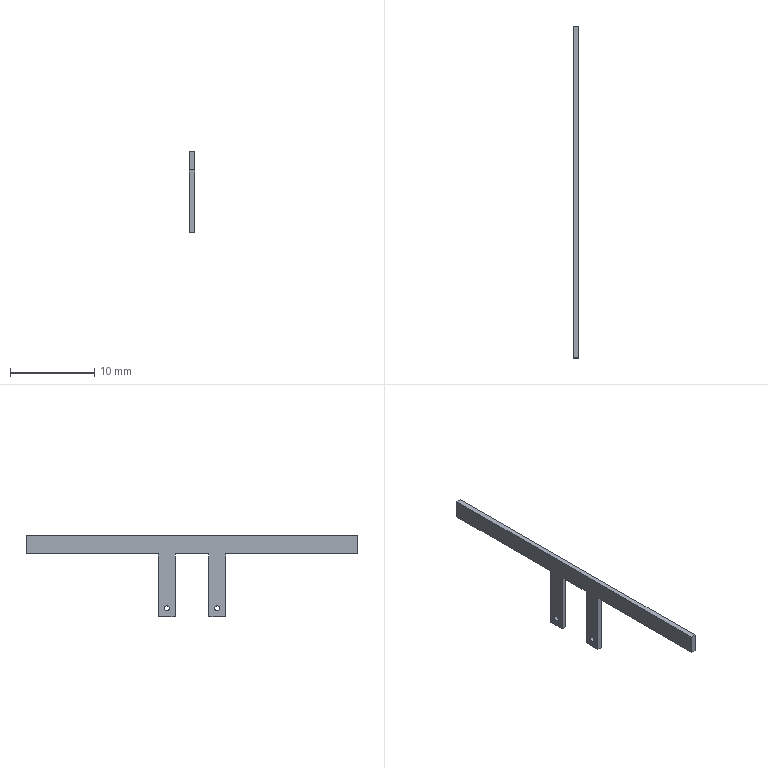Part | NX | features DATUM_CSYS 3, SIMPLE HOLE 2, SKETCH 2, EXTRUDE 1, HOLE PACKAGE 1 | 1 solid | 16 faces | box 0.6 x 39.5 x 9.68 mm | volume 70.179 mm3 | plane 14 | cylinder 2 | commonest cylinder face diameters 0.6 x2
STEP:
#1=CARTESIAN_POINT('',(0.,-19.75,2.22));
#2=VERTEX_POINT('',#1);
#3=CARTESIAN_POINT('',(0.,-19.75,0.));
#4=VERTEX_POINT('',#3);
#5=CARTESIAN_POINT('',(0.,-19.75,2.22));
#6=DIRECTION('',(0.,0.,-1.));
#7=VECTOR('',#6,1000.);
#8=LINE('',#5,#7);
#9=EDGE_CURVE('',#2,#4,#8,.T.);
#10=ORIENTED_EDGE('',*,*,#9,.T.);
#11=CARTESIAN_POINT('',(0.6,-19.75,0.));
#12=VERTEX_POINT('',#11);
#13=CARTESIAN_POINT('',(0.6,-19.75,0.));
#14=DIRECTION('',(-1.,0.,0.));
#15=VECTOR('',#14,1000.);
#16=LINE('',#13,#15);
#17=EDGE_CURVE('',#12,#4,#16,.T.);
#18=ORIENTED_EDGE('',*,*,#17,.F.);
#19=CARTESIAN_POINT('',(0.6,-19.75,2.22));
#20=VERTEX_POINT('',#19);
#21=CARTESIAN_POINT('',(0.6,-19.75,2.22));
#22=DIRECTION('',(0.,0.,-1.));
#23=VECTOR('',#22,1000.);
#24=LINE('',#21,#23);
#25=EDGE_CURVE('',#20,#12,#24,.T.);
#26=ORIENTED_EDGE('',*,*,#25,.F.);
#27=CARTESIAN_POINT('',(0.6,-19.75,2.22));
#28=DIRECTION('',(-1.,0.,0.));
#29=VECTOR('',#28,1000.);
#30=LINE('',#27,#29);
#31=EDGE_CURVE('',#20,#2,#30,.T.);
#32=ORIENTED_EDGE('',*,*,#31,.T.);
#33=EDGE_LOOP('',(#10,#18,#26,#32));
#34=FACE_BOUND('',#33,.T.);
#35=CARTESIAN_POINT('',(0.6,-19.75,2.22));
#36=DIRECTION('',(0.,1.,0.));
#37=DIRECTION('',(0.,0.,1.));
#38=AXIS2_PLACEMENT_3D('',#35,#36,#37);
#39=PLANE('',#38);
#40=ADVANCED_FACE('',(#34),#39,.F.);
#41=CARTESIAN_POINT('',(0.,-4.,0.));
#42=VERTEX_POINT('',#41);
#43=CARTESIAN_POINT('',(0.,-19.75,0.));
#44=DIRECTION('',(0.,1.,0.));
#45=VECTOR('',#44,1000.);
#46=LINE('',#43,#45);
#47=EDGE_CURVE('',#4,#42,#46,.T.);
#48=ORIENTED_EDGE('',*,*,#47,.T.);
#49=CARTESIAN_POINT('',(0.6,-4.,0.));
#50=VERTEX_POINT('',#49);
#51=CARTESIAN_POINT('',(0.6,-4.,0.));
#52=DIRECTION('',(-1.,0.,0.));
#53=VECTOR('',#52,1000.);
#54=LINE('',#51,#53);
#55=EDGE_CURVE('',#50,#42,#54,.T.);
#56=ORIENTED_EDGE('',*,*,#55,.F.);
#57=CARTESIAN_POINT('',(0.6,-19.75,0.));
#58=DIRECTION('',(0.,1.,0.));
#59=VECTOR('',#58,1000.);
#60=LINE('',#57,#59);
#61=EDGE_CURVE('',#12,#50,#60,.T.);
#62=ORIENTED_EDGE('',*,*,#61,.F.);
#63=ORIENTED_EDGE('',*,*,#17,.T.);
#64=EDGE_LOOP('',(#48,#56,#62,#63));
#65=FACE_BOUND('',#64,.T.);
#66=CARTESIAN_POINT('',(0.6,-19.75,0.));
#67=DIRECTION('',(0.,0.,1.));
#68=DIRECTION('',(1.,0.,0.));
#69=AXIS2_PLACEMENT_3D('',#66,#67,#68);
#70=PLANE('',#69);
#71=ADVANCED_FACE('',(#65),#70,.F.);
#72=CARTESIAN_POINT('',(0.,-4.,-7.46));
#73=VERTEX_POINT('',#72);
#74=CARTESIAN_POINT('',(0.,-4.,0.));
#75=DIRECTION('',(0.,0.,-1.));
#76=VECTOR('',#75,1000.);
#77=LINE('',#74,#76);
#78=EDGE_CURVE('',#42,#73,#77,.T.);
#79=ORIENTED_EDGE('',*,*,#78,.T.);
#80=CARTESIAN_POINT('',(0.6,-4.,-7.46));
#81=VERTEX_POINT('',#80);
#82=CARTESIAN_POINT('',(0.6,-4.,-7.46));
#83=DIRECTION('',(-1.,0.,0.));
#84=VECTOR('',#83,1000.);
#85=LINE('',#82,#84);
#86=EDGE_CURVE('',#81,#73,#85,.T.);
#87=ORIENTED_EDGE('',*,*,#86,.F.);
#88=CARTESIAN_POINT('',(0.6,-4.,0.));
#89=DIRECTION('',(0.,0.,-1.));
#90=VECTOR('',#89,1000.);
#91=LINE('',#88,#90);
#92=EDGE_CURVE('',#50,#81,#91,.T.);
#93=ORIENTED_EDGE('',*,*,#92,.F.);
#94=ORIENTED_EDGE('',*,*,#55,.T.);
#95=EDGE_LOOP('',(#79,#87,#93,#94));
#96=FACE_BOUND('',#95,.T.);
#97=CARTESIAN_POINT('',(0.6,-4.,0.));
#98=DIRECTION('',(0.,1.,0.));
#99=DIRECTION('',(0.,0.,1.));
#100=AXIS2_PLACEMENT_3D('',#97,#98,#99);
#101=PLANE('',#100);
#102=ADVANCED_FACE('',(#96),#101,.F.);
#103=CARTESIAN_POINT('',(0.,-2.,-7.46));
#104=VERTEX_POINT('',#103);
#105=CARTESIAN_POINT('',(0.,-4.,-7.46));
#106=DIRECTION('',(0.,1.,0.));
#107=VECTOR('',#106,1000.);
#108=LINE('',#105,#107);
#109=EDGE_CURVE('',#73,#104,#108,.T.);
#110=ORIENTED_EDGE('',*,*,#109,.T.);
#111=CARTESIAN_POINT('',(0.6,-2.,-7.46));
#112=VERTEX_POINT('',#111);
#113=CARTESIAN_POINT('',(0.6,-2.,-7.46));
#114=DIRECTION('',(-1.,0.,0.));
#115=VECTOR('',#114,1000.);
#116=LINE('',#113,#115);
#117=EDGE_CURVE('',#112,#104,#116,.T.);
#118=ORIENTED_EDGE('',*,*,#117,.F.);
#119=CARTESIAN_POINT('',(0.6,-4.,-7.46));
#120=DIRECTION('',(0.,1.,0.));
#121=VECTOR('',#120,1000.);
#122=LINE('',#119,#121);
#123=EDGE_CURVE('',#81,#112,#122,.T.);
#124=ORIENTED_EDGE('',*,*,#123,.F.);
#125=ORIENTED_EDGE('',*,*,#86,.T.);
#126=EDGE_LOOP('',(#110,#118,#124,#125));
#127=FACE_BOUND('',#126,.T.);
#128=CARTESIAN_POINT('',(0.6,-4.,-7.46));
#129=DIRECTION('',(0.,0.,1.));
#130=DIRECTION('',(0.,-1.,0.));
#131=AXIS2_PLACEMENT_3D('',#128,#129,#130);
#132=PLANE('',#131);
#133=ADVANCED_FACE('',(#127),#132,.F.);
#134=CARTESIAN_POINT('',(0.,-2.,0.));
#135=VERTEX_POINT('',#134);
#136=CARTESIAN_POINT('',(0.,-2.,-7.46));
#137=DIRECTION('',(0.,0.,1.));
#138=VECTOR('',#137,1000.);
#139=LINE('',#136,#138);
#140=EDGE_CURVE('',#104,#135,#139,.T.);
#141=ORIENTED_EDGE('',*,*,#140,.T.);
#142=CARTESIAN_POINT('',(0.6,-2.,0.));
#143=VERTEX_POINT('',#142);
#144=CARTESIAN_POINT('',(0.6,-2.,0.));
#145=DIRECTION('',(-1.,0.,0.));
#146=VECTOR('',#145,1000.);
#147=LINE('',#144,#146);
#148=EDGE_CURVE('',#143,#135,#147,.T.);
#149=ORIENTED_EDGE('',*,*,#148,.F.);
#150=CARTESIAN_POINT('',(0.6,-2.,-7.46));
#151=DIRECTION('',(0.,0.,1.));
#152=VECTOR('',#151,1000.);
#153=LINE('',#150,#152);
#154=EDGE_CURVE('',#112,#143,#153,.T.);
#155=ORIENTED_EDGE('',*,*,#154,.F.);
#156=ORIENTED_EDGE('',*,*,#117,.T.);
#157=EDGE_LOOP('',(#141,#149,#155,#156));
#158=FACE_BOUND('',#157,.T.);
#159=CARTESIAN_POINT('',(0.6,-2.,-7.46));
#160=DIRECTION('',(0.,-1.,0.));
#161=DIRECTION('',(0.,0.,-1.));
#162=AXIS2_PLACEMENT_3D('',#159,#160,#161);
#163=PLANE('',#162);
#164=ADVANCED_FACE('',(#158),#163,.F.);
#165=CARTESIAN_POINT('',(0.,2.,0.));
#166=VERTEX_POINT('',#165);
#167=CARTESIAN_POINT('',(0.,-2.,0.));
#168=DIRECTION('',(0.,1.,0.));
#169=VECTOR('',#168,1000.);
#170=LINE('',#167,#169);
#171=EDGE_CURVE('',#135,#166,#170,.T.);
#172=ORIENTED_EDGE('',*,*,#171,.T.);
#173=CARTESIAN_POINT('',(0.6,2.,0.));
#174=VERTEX_POINT('',#173);
#175=CARTESIAN_POINT('',(0.6,2.,0.));
#176=DIRECTION('',(-1.,0.,0.));
#177=VECTOR('',#176,1000.);
#178=LINE('',#175,#177);
#179=EDGE_CURVE('',#174,#166,#178,.T.);
#180=ORIENTED_EDGE('',*,*,#179,.F.);
#181=CARTESIAN_POINT('',(0.6,-2.,0.));
#182=DIRECTION('',(0.,1.,0.));
#183=VECTOR('',#182,1000.);
#184=LINE('',#181,#183);
#185=EDGE_CURVE('',#143,#174,#184,.T.);
#186=ORIENTED_EDGE('',*,*,#185,.F.);
#187=ORIENTED_EDGE('',*,*,#148,.T.);
#188=EDGE_LOOP('',(#172,#180,#186,#187));
#189=FACE_BOUND('',#188,.T.);
#190=CARTESIAN_POINT('',(0.6,-2.,0.));
#191=DIRECTION('',(0.,0.,1.));
#192=DIRECTION('',(1.,0.,0.));
#193=AXIS2_PLACEMENT_3D('',#190,#191,#192);
#194=PLANE('',#193);
#195=ADVANCED_FACE('',(#189),#194,.F.);
#196=CARTESIAN_POINT('',(0.,2.,-7.46));
#197=VERTEX_POINT('',#196);
#198=CARTESIAN_POINT('',(0.,2.,0.));
#199=DIRECTION('',(0.,0.,-1.));
#200=VECTOR('',#199,1000.);
#201=LINE('',#198,#200);
#202=EDGE_CURVE('',#166,#197,#201,.T.);
#203=ORIENTED_EDGE('',*,*,#202,.T.);
#204=CARTESIAN_POINT('',(0.6,2.,-7.46));
#205=VERTEX_POINT('',#204);
#206=CARTESIAN_POINT('',(0.6,2.,-7.46));
#207=DIRECTION('',(-1.,0.,0.));
#208=VECTOR('',#207,1000.);
#209=LINE('',#206,#208);
#210=EDGE_CURVE('',#205,#197,#209,.T.);
#211=ORIENTED_EDGE('',*,*,#210,.F.);
#212=CARTESIAN_POINT('',(0.6,2.,0.));
#213=DIRECTION('',(0.,0.,-1.));
#214=VECTOR('',#213,1000.);
#215=LINE('',#212,#214);
#216=EDGE_CURVE('',#174,#205,#215,.T.);
#217=ORIENTED_EDGE('',*,*,#216,.F.);
#218=ORIENTED_EDGE('',*,*,#179,.T.);
#219=EDGE_LOOP('',(#203,#211,#217,#218));
#220=FACE_BOUND('',#219,.T.);
#221=CARTESIAN_POINT('',(0.6,2.,0.));
#222=DIRECTION('',(0.,1.,0.));
#223=DIRECTION('',(0.,0.,1.));
#224=AXIS2_PLACEMENT_3D('',#221,#222,#223);
#225=PLANE('',#224);
#226=ADVANCED_FACE('',(#220),#225,.F.);
#227=CARTESIAN_POINT('',(0.,4.,-7.46));
#228=VERTEX_POINT('',#227);
#229=CARTESIAN_POINT('',(0.,2.,-7.46));
#230=DIRECTION('',(0.,1.,0.));
#231=VECTOR('',#230,1000.);
#232=LINE('',#229,#231);
#233=EDGE_CURVE('',#197,#228,#232,.T.);
#234=ORIENTED_EDGE('',*,*,#233,.T.);
#235=CARTESIAN_POINT('',(0.6,4.,-7.46));
#236=VERTEX_POINT('',#235);
#237=CARTESIAN_POINT('',(0.6,4.,-7.46));
#238=DIRECTION('',(-1.,0.,0.));
#239=VECTOR('',#238,1000.);
#240=LINE('',#237,#239);
#241=EDGE_CURVE('',#236,#228,#240,.T.);
#242=ORIENTED_EDGE('',*,*,#241,.F.);
#243=CARTESIAN_POINT('',(0.6,2.,-7.46));
#244=DIRECTION('',(0.,1.,0.));
#245=VECTOR('',#244,1000.);
#246=LINE('',#243,#245);
#247=EDGE_CURVE('',#205,#236,#246,.T.);
#248=ORIENTED_EDGE('',*,*,#247,.F.);
#249=ORIENTED_EDGE('',*,*,#210,.T.);
#250=EDGE_LOOP('',(#234,#242,#248,#249));
#251=FACE_BOUND('',#250,.T.);
#252=CARTESIAN_POINT('',(0.6,2.,-7.46));
#253=DIRECTION('',(0.,0.,1.));
#254=DIRECTION('',(0.,-1.,0.));
#255=AXIS2_PLACEMENT_3D('',#252,#253,#254);
#256=PLANE('',#255);
#257=ADVANCED_FACE('',(#251),#256,.F.);
#258=CARTESIAN_POINT('',(0.,4.,0.));
#259=VERTEX_POINT('',#258);
#260=CARTESIAN_POINT('',(0.,4.,-7.46));
#261=DIRECTION('',(0.,0.,1.));
#262=VECTOR('',#261,1000.);
#263=LINE('',#260,#262);
#264=EDGE_CURVE('',#228,#259,#263,.T.);
#265=ORIENTED_EDGE('',*,*,#264,.T.);
#266=CARTESIAN_POINT('',(0.6,4.,0.));
#267=VERTEX_POINT('',#266);
#268=CARTESIAN_POINT('',(0.6,4.,0.));
#269=DIRECTION('',(-1.,0.,0.));
#270=VECTOR('',#269,1000.);
#271=LINE('',#268,#270);
#272=EDGE_CURVE('',#267,#259,#271,.T.);
#273=ORIENTED_EDGE('',*,*,#272,.F.);
#274=CARTESIAN_POINT('',(0.6,4.,-7.46));
#275=DIRECTION('',(0.,0.,1.));
#276=VECTOR('',#275,1000.);
#277=LINE('',#274,#276);
#278=EDGE_CURVE('',#236,#267,#277,.T.);
#279=ORIENTED_EDGE('',*,*,#278,.F.);
#280=ORIENTED_EDGE('',*,*,#241,.T.);
#281=EDGE_LOOP('',(#265,#273,#279,#280));
#282=FACE_BOUND('',#281,.T.);
#283=CARTESIAN_POINT('',(0.6,4.,-7.46));
#284=DIRECTION('',(0.,-1.,0.));
#285=DIRECTION('',(0.,0.,-1.));
#286=AXIS2_PLACEMENT_3D('',#283,#284,#285);
#287=PLANE('',#286);
#288=ADVANCED_FACE('',(#282),#287,.F.);
#289=CARTESIAN_POINT('',(0.,19.75,0.));
#290=VERTEX_POINT('',#289);
#291=CARTESIAN_POINT('',(0.,4.,0.));
#292=DIRECTION('',(0.,1.,0.));
#293=VECTOR('',#292,1000.);
#294=LINE('',#291,#293);
#295=EDGE_CURVE('',#259,#290,#294,.T.);
#296=ORIENTED_EDGE('',*,*,#295,.T.);
#297=CARTESIAN_POINT('',(0.6,19.75,0.));
#298=VERTEX_POINT('',#297);
#299=CARTESIAN_POINT('',(0.6,19.75,0.));
#300=DIRECTION('',(-1.,0.,0.));
#301=VECTOR('',#300,1000.);
#302=LINE('',#299,#301);
#303=EDGE_CURVE('',#298,#290,#302,.T.);
#304=ORIENTED_EDGE('',*,*,#303,.F.);
#305=CARTESIAN_POINT('',(0.6,4.,0.));
#306=DIRECTION('',(0.,1.,0.));
#307=VECTOR('',#306,1000.);
#308=LINE('',#305,#307);
#309=EDGE_CURVE('',#267,#298,#308,.T.);
#310=ORIENTED_EDGE('',*,*,#309,.F.);
#311=ORIENTED_EDGE('',*,*,#272,.T.);
#312=EDGE_LOOP('',(#296,#304,#310,#311));
#313=FACE_BOUND('',#312,.T.);
#314=CARTESIAN_POINT('',(0.6,4.,0.));
#315=DIRECTION('',(0.,0.,1.));
#316=DIRECTION('',(1.,0.,0.));
#317=AXIS2_PLACEMENT_3D('',#314,#315,#316);
#318=PLANE('',#317);
#319=ADVANCED_FACE('',(#313),#318,.F.);
#320=CARTESIAN_POINT('',(0.,19.75,2.22));
#321=VERTEX_POINT('',#320);
#322=CARTESIAN_POINT('',(0.,19.75,0.));
#323=DIRECTION('',(0.,0.,1.));
#324=VECTOR('',#323,1000.);
#325=LINE('',#322,#324);
#326=EDGE_CURVE('',#290,#321,#325,.T.);
#327=ORIENTED_EDGE('',*,*,#326,.T.);
#328=CARTESIAN_POINT('',(0.6,19.75,2.22));
#329=VERTEX_POINT('',#328);
#330=CARTESIAN_POINT('',(0.6,19.75,2.22));
#331=DIRECTION('',(-1.,0.,0.));
#332=VECTOR('',#331,1000.);
#333=LINE('',#330,#332);
#334=EDGE_CURVE('',#329,#321,#333,.T.);
#335=ORIENTED_EDGE('',*,*,#334,.F.);
#336=CARTESIAN_POINT('',(0.6,19.75,0.));
#337=DIRECTION('',(0.,0.,1.));
#338=VECTOR('',#337,1000.);
#339=LINE('',#336,#338);
#340=EDGE_CURVE('',#298,#329,#339,.T.);
#341=ORIENTED_EDGE('',*,*,#340,.F.);
#342=ORIENTED_EDGE('',*,*,#303,.T.);
#343=EDGE_LOOP('',(#327,#335,#341,#342));
#344=FACE_BOUND('',#343,.T.);
#345=CARTESIAN_POINT('',(0.6,19.75,0.));
#346=DIRECTION('',(0.,-1.,0.));
#347=DIRECTION('',(0.,0.,-1.));
#348=AXIS2_PLACEMENT_3D('',#345,#346,#347);
#349=PLANE('',#348);
#350=ADVANCED_FACE('',(#344),#349,.F.);
#351=CARTESIAN_POINT('',(0.,19.75,2.22));
#352=DIRECTION('',(0.,-1.,0.));
#353=VECTOR('',#352,1000.);
#354=LINE('',#351,#353);
#355=EDGE_CURVE('',#321,#2,#354,.T.);
#356=ORIENTED_EDGE('',*,*,#355,.T.);
#357=ORIENTED_EDGE('',*,*,#31,.F.);
#358=CARTESIAN_POINT('',(0.6,19.75,2.22));
#359=DIRECTION('',(0.,-1.,0.));
#360=VECTOR('',#359,1000.);
#361=LINE('',#358,#360);
#362=EDGE_CURVE('',#329,#20,#361,.T.);
#363=ORIENTED_EDGE('',*,*,#362,.F.);
#364=ORIENTED_EDGE('',*,*,#334,.T.);
#365=EDGE_LOOP('',(#356,#357,#363,#364));
#366=FACE_BOUND('',#365,.T.);
#367=CARTESIAN_POINT('',(0.6,19.75,2.22));
#368=DIRECTION('',(0.,0.,-1.));
#369=DIRECTION('',(-1.,0.,0.));
#370=AXIS2_PLACEMENT_3D('',#367,#368,#369);
#371=PLANE('',#370);
#372=ADVANCED_FACE('',(#366),#371,.F.);
#373=CARTESIAN_POINT('',(0.6,3.,-6.16));
#374=VERTEX_POINT('',#373);
#375=CARTESIAN_POINT('',(0.6,3.,-6.46));
#376=DIRECTION('',(-1.,0.,0.));
#377=DIRECTION('',(0.,0.,1.));
#378=AXIS2_PLACEMENT_3D('',#375,#376,#377);
#379=CIRCLE('',#378,0.3);
#380=EDGE_CURVE('',#374,#374,#379,.T.);
#381=ORIENTED_EDGE('',*,*,#380,.T.);
#382=EDGE_LOOP('',(#381));
#383=FACE_BOUND('',#382,.T.);
#384=CARTESIAN_POINT('',(0.6,-3.,-6.16));
#385=VERTEX_POINT('',#384);
#386=CARTESIAN_POINT('',(0.6,-3.,-6.46));
#387=DIRECTION('',(-1.,0.,0.));
#388=DIRECTION('',(0.,0.,1.));
#389=AXIS2_PLACEMENT_3D('',#386,#387,#388);
#390=CIRCLE('',#389,0.3);
#391=EDGE_CURVE('',#385,#385,#390,.T.);
#392=ORIENTED_EDGE('',*,*,#391,.T.);
#393=EDGE_LOOP('',(#392));
#394=FACE_BOUND('',#393,.T.);
#395=ORIENTED_EDGE('',*,*,#25,.T.);
#396=ORIENTED_EDGE('',*,*,#61,.T.);
#397=ORIENTED_EDGE('',*,*,#92,.T.);
#398=ORIENTED_EDGE('',*,*,#123,.T.);
#399=ORIENTED_EDGE('',*,*,#154,.T.);
#400=ORIENTED_EDGE('',*,*,#185,.T.);
#401=ORIENTED_EDGE('',*,*,#216,.T.);
#402=ORIENTED_EDGE('',*,*,#247,.T.);
#403=ORIENTED_EDGE('',*,*,#278,.T.);
#404=ORIENTED_EDGE('',*,*,#309,.T.);
#405=ORIENTED_EDGE('',*,*,#340,.T.);
#406=ORIENTED_EDGE('',*,*,#362,.T.);
#407=EDGE_LOOP('',(#395,#396,#397,#398,#399,#400,#401,#402,#403,#404,#405,#406));
#408=FACE_BOUND('',#407,.T.);
#409=CARTESIAN_POINT('',(0.6,0.,0.));
#410=DIRECTION('',(1.,0.,0.));
#411=DIRECTION('',(0.,0.,-1.));
#412=AXIS2_PLACEMENT_3D('',#409,#410,#411);
#413=PLANE('',#412);
#414=ADVANCED_FACE('',(#383,#394,#408),#413,.T.);
#415=CARTESIAN_POINT('',(0.,3.,-6.76));
#416=VERTEX_POINT('',#415);
#417=CARTESIAN_POINT('',(0.,3.,-6.46));
#418=DIRECTION('',(1.,0.,0.));
#419=DIRECTION('',(0.,0.,-1.));
#420=AXIS2_PLACEMENT_3D('',#417,#418,#419);
#421=CIRCLE('',#420,0.3);
#422=EDGE_CURVE('',#416,#416,#421,.T.);
#423=ORIENTED_EDGE('',*,*,#422,.T.);
#424=EDGE_LOOP('',(#423));
#425=FACE_BOUND('',#424,.T.);
#426=CARTESIAN_POINT('',(0.,-3.,-6.76));
#427=VERTEX_POINT('',#426);
#428=CARTESIAN_POINT('',(0.,-3.,-6.46));
#429=DIRECTION('',(1.,0.,0.));
#430=DIRECTION('',(0.,0.,-1.));
#431=AXIS2_PLACEMENT_3D('',#428,#429,#430);
#432=CIRCLE('',#431,0.3);
#433=EDGE_CURVE('',#427,#427,#432,.T.);
#434=ORIENTED_EDGE('',*,*,#433,.T.);
#435=EDGE_LOOP('',(#434));
#436=FACE_BOUND('',#435,.T.);
#437=ORIENTED_EDGE('',*,*,#9,.F.);
#438=ORIENTED_EDGE('',*,*,#355,.F.);
#439=ORIENTED_EDGE('',*,*,#326,.F.);
#440=ORIENTED_EDGE('',*,*,#295,.F.);
#441=ORIENTED_EDGE('',*,*,#264,.F.);
#442=ORIENTED_EDGE('',*,*,#233,.F.);
#443=ORIENTED_EDGE('',*,*,#202,.F.);
#444=ORIENTED_EDGE('',*,*,#171,.F.);
#445=ORIENTED_EDGE('',*,*,#140,.F.);
#446=ORIENTED_EDGE('',*,*,#109,.F.);
#447=ORIENTED_EDGE('',*,*,#78,.F.);
#448=ORIENTED_EDGE('',*,*,#47,.F.);
#449=EDGE_LOOP('',(#437,#438,#439,#440,#441,#442,#443,#444,#445,#446,#447,#448));
#450=FACE_BOUND('',#449,.T.);
#451=CARTESIAN_POINT('',(0.,0.,0.));
#452=DIRECTION('',(1.,0.,0.));
#453=DIRECTION('',(0.,0.,-1.));
#454=AXIS2_PLACEMENT_3D('',#451,#452,#453);
#455=PLANE('',#454);
#456=ADVANCED_FACE('',(#425,#436,#450),#455,.F.);
#457=ORIENTED_EDGE('',*,*,#391,.F.);
#458=EDGE_LOOP('',(#457));
#459=FACE_BOUND('',#458,.T.);
#460=ORIENTED_EDGE('',*,*,#433,.F.);
#461=EDGE_LOOP('',(#460));
#462=FACE_BOUND('',#461,.T.);
#463=CARTESIAN_POINT('',(0.6,-3.,-6.46));
#464=DIRECTION('',(-1.,0.,0.));
#465=DIRECTION('',(0.,0.,1.));
#466=AXIS2_PLACEMENT_3D('',#463,#464,#465);
#467=CYLINDRICAL_SURFACE('',#466,0.3);
#468=ADVANCED_FACE('',(#459,#462),#467,.F.);
#469=ORIENTED_EDGE('',*,*,#380,.F.);
#470=EDGE_LOOP('',(#469));
#471=FACE_BOUND('',#470,.T.);
#472=ORIENTED_EDGE('',*,*,#422,.F.);
#473=EDGE_LOOP('',(#472));
#474=FACE_BOUND('',#473,.T.);
#475=CARTESIAN_POINT('',(0.6,3.,-6.46));
#476=DIRECTION('',(-1.,0.,0.));
#477=DIRECTION('',(0.,0.,1.));
#478=AXIS2_PLACEMENT_3D('',#475,#476,#477);
#479=CYLINDRICAL_SURFACE('',#478,0.3);
#480=ADVANCED_FACE('',(#471,#474),#479,.F.);
#481=CLOSED_SHELL('',(#40,#71,#102,#133,#164,#195,#226,#257,#288,#319,#350,#372,#414,#456,#468,#480));
#482=MANIFOLD_SOLID_BREP('',#481);
#483=(LENGTH_UNIT()NAMED_UNIT(*)SI_UNIT(.MILLI.,.METRE.));
#484=UNCERTAINTY_MEASURE_WITH_UNIT(LENGTH_MEASURE(0.00001),#483,'','');
#485=(NAMED_UNIT(*)PLANE_ANGLE_UNIT()SI_UNIT($,.RADIAN.));
#486=(NAMED_UNIT(*)SI_UNIT($,.STERADIAN.)SOLID_ANGLE_UNIT());
#487=(GEOMETRIC_REPRESENTATION_CONTEXT(3)GLOBAL_UNCERTAINTY_ASSIGNED_CONTEXT((#484))GLOBAL_UNIT_ASSIGNED_CONTEXT((#483,#485,#486))REPRESENTATION_CONTEXT('',''));
#488=ADVANCED_BREP_SHAPE_REPRESENTATION('',(#482),#487);